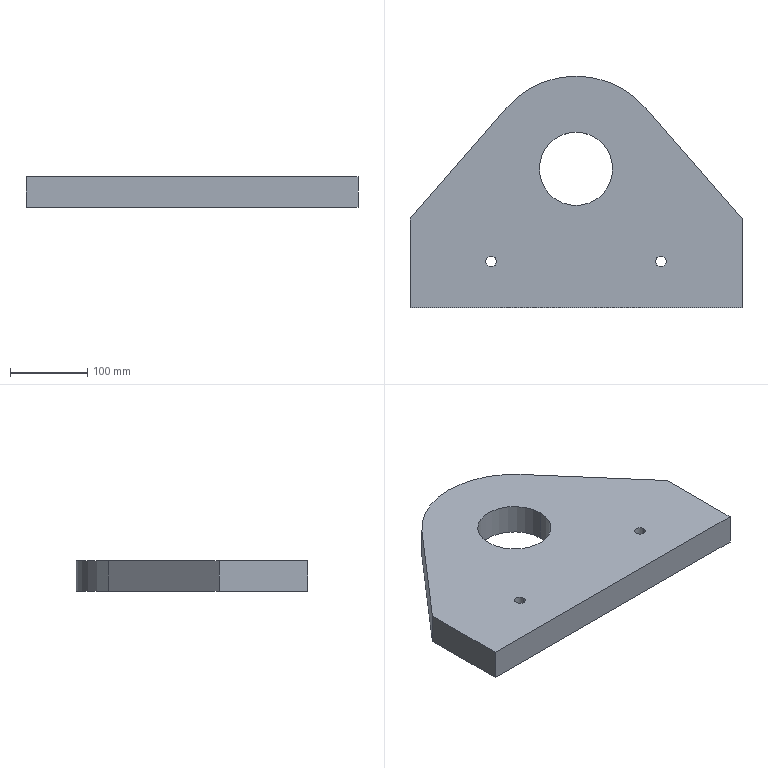Part | SolidWorks | features Extrusion 1, HoleWzd 1, ICE 1 | 1 solid | 14 faces | box 430 x 300 x 40 mm | volume 3646282 mm3 | cylinder 7 | plane 7 | commonest cylinder face diameters 14 x4 95 x2 240 x1
STEP:
#1=CARTESIAN_POINT('',(-117.,-120.,0.));
#2=VERTEX_POINT('',#1);
#3=CARTESIAN_POINT('',(-103.,-120.,0.));
#4=VERTEX_POINT('',#3);
#5=CARTESIAN_POINT('',(-110.,-120.,0.));
#6=DIRECTION('',(0.,0.,1.));
#7=DIRECTION('',(1.,0.,0.));
#8=AXIS2_PLACEMENT_3D('',#5,#6,#7);
#9=CIRCLE('',#8,7.);
#10=EDGE_CURVE('',#2,#4,#9,.T.);
#11=ORIENTED_EDGE('',*,*,#10,.F.);
#12=CARTESIAN_POINT('',(-117.,-120.,40.));
#13=VERTEX_POINT('',#12);
#14=CARTESIAN_POINT('',(-117.,-120.,40.));
#15=DIRECTION('',(0.,0.,1.));
#16=VECTOR('',#15,1000.);
#17=LINE('',#14,#16);
#18=EDGE_CURVE('',#2,#13,#17,.T.);
#19=ORIENTED_EDGE('',*,*,#18,.T.);
#20=CARTESIAN_POINT('',(-103.,-120.,40.));
#21=VERTEX_POINT('',#20);
#22=CARTESIAN_POINT('',(-110.,-120.,40.));
#23=DIRECTION('',(0.,0.,1.));
#24=DIRECTION('',(1.,0.,0.));
#25=AXIS2_PLACEMENT_3D('',#22,#23,#24);
#26=CIRCLE('',#25,7.);
#27=EDGE_CURVE('',#13,#21,#26,.T.);
#28=ORIENTED_EDGE('',*,*,#27,.T.);
#29=CARTESIAN_POINT('',(-103.,-120.,40.));
#30=DIRECTION('',(0.,0.,1.));
#31=VECTOR('',#30,1000.);
#32=LINE('',#29,#31);
#33=EDGE_CURVE('',#4,#21,#32,.T.);
#34=ORIENTED_EDGE('',*,*,#33,.F.);
#35=EDGE_LOOP('',(#11,#19,#28,#34));
#36=FACE_OUTER_BOUND('',#35,.T.);
#37=CARTESIAN_POINT('',(-110.,-120.,40.));
#38=DIRECTION('',(0.,0.,1.));
#39=DIRECTION('',(1.,0.,0.));
#40=AXIS2_PLACEMENT_3D('',#37,#38,#39);
#41=CYLINDRICAL_SURFACE('',#40,7.);
#42=ADVANCED_FACE('',(#36),#41,.F.);
#43=CARTESIAN_POINT('',(103.,-120.,0.));
#44=VERTEX_POINT('',#43);
#45=CARTESIAN_POINT('',(117.,-120.,0.));
#46=VERTEX_POINT('',#45);
#47=CARTESIAN_POINT('',(110.,-120.,0.));
#48=DIRECTION('',(0.,0.,1.));
#49=DIRECTION('',(1.,0.,0.));
#50=AXIS2_PLACEMENT_3D('',#47,#48,#49);
#51=CIRCLE('',#50,7.);
#52=EDGE_CURVE('',#44,#46,#51,.T.);
#53=ORIENTED_EDGE('',*,*,#52,.F.);
#54=CARTESIAN_POINT('',(103.,-120.,40.));
#55=VERTEX_POINT('',#54);
#56=CARTESIAN_POINT('',(103.,-120.,40.));
#57=DIRECTION('',(0.,0.,1.));
#58=VECTOR('',#57,1000.);
#59=LINE('',#56,#58);
#60=EDGE_CURVE('',#44,#55,#59,.T.);
#61=ORIENTED_EDGE('',*,*,#60,.T.);
#62=CARTESIAN_POINT('',(117.,-120.,40.));
#63=VERTEX_POINT('',#62);
#64=CARTESIAN_POINT('',(110.,-120.,40.));
#65=DIRECTION('',(0.,0.,1.));
#66=DIRECTION('',(1.,0.,0.));
#67=AXIS2_PLACEMENT_3D('',#64,#65,#66);
#68=CIRCLE('',#67,7.);
#69=EDGE_CURVE('',#55,#63,#68,.T.);
#70=ORIENTED_EDGE('',*,*,#69,.T.);
#71=CARTESIAN_POINT('',(117.,-120.,40.));
#72=DIRECTION('',(0.,0.,1.));
#73=VECTOR('',#72,1000.);
#74=LINE('',#71,#73);
#75=EDGE_CURVE('',#46,#63,#74,.T.);
#76=ORIENTED_EDGE('',*,*,#75,.F.);
#77=EDGE_LOOP('',(#53,#61,#70,#76));
#78=FACE_OUTER_BOUND('',#77,.T.);
#79=CARTESIAN_POINT('',(110.,-120.,40.));
#80=DIRECTION('',(0.,0.,1.));
#81=DIRECTION('',(1.,0.,0.));
#82=AXIS2_PLACEMENT_3D('',#79,#80,#81);
#83=CYLINDRICAL_SURFACE('',#82,7.);
#84=ADVANCED_FACE('',(#78),#83,.F.);
#85=CARTESIAN_POINT('',(-47.5,0.,0.));
#86=VERTEX_POINT('',#85);
#87=CARTESIAN_POINT('',(47.5,0.,0.));
#88=VERTEX_POINT('',#87);
#89=CARTESIAN_POINT('',(0.,0.,0.));
#90=DIRECTION('',(0.,0.,1.));
#91=DIRECTION('',(1.,0.,0.));
#92=AXIS2_PLACEMENT_3D('',#89,#90,#91);
#93=CIRCLE('',#92,47.5);
#94=EDGE_CURVE('',#86,#88,#93,.T.);
#95=ORIENTED_EDGE('',*,*,#94,.F.);
#96=CARTESIAN_POINT('',(-47.5,0.,40.));
#97=VERTEX_POINT('',#96);
#98=CARTESIAN_POINT('',(-47.5,0.,0.));
#99=DIRECTION('',(0.,0.,1.));
#100=VECTOR('',#99,1000.);
#101=LINE('',#98,#100);
#102=EDGE_CURVE('',#86,#97,#101,.T.);
#103=ORIENTED_EDGE('',*,*,#102,.T.);
#104=CARTESIAN_POINT('',(47.5,0.,40.));
#105=VERTEX_POINT('',#104);
#106=CARTESIAN_POINT('',(0.,0.,40.));
#107=DIRECTION('',(0.,0.,1.));
#108=DIRECTION('',(1.,0.,0.));
#109=AXIS2_PLACEMENT_3D('',#106,#107,#108);
#110=CIRCLE('',#109,47.5);
#111=EDGE_CURVE('',#97,#105,#110,.T.);
#112=ORIENTED_EDGE('',*,*,#111,.T.);
#113=CARTESIAN_POINT('',(47.5,0.,0.));
#114=DIRECTION('',(0.,0.,1.));
#115=VECTOR('',#114,1000.);
#116=LINE('',#113,#115);
#117=EDGE_CURVE('',#88,#105,#116,.T.);
#118=ORIENTED_EDGE('',*,*,#117,.F.);
#119=EDGE_LOOP('',(#95,#103,#112,#118));
#120=FACE_OUTER_BOUND('',#119,.T.);
#121=CARTESIAN_POINT('',(0.,0.,0.));
#122=DIRECTION('',(0.,0.,1.));
#123=DIRECTION('',(1.,0.,0.));
#124=AXIS2_PLACEMENT_3D('',#121,#122,#123);
#125=CYLINDRICAL_SURFACE('',#124,47.5);
#126=ADVANCED_FACE('',(#120),#125,.F.);
#127=CARTESIAN_POINT('',(90.723,78.545,0.));
#128=VERTEX_POINT('',#127);
#129=CARTESIAN_POINT('',(215.,-65.,0.));
#130=VERTEX_POINT('',#129);
#131=CARTESIAN_POINT('',(90.723,78.545,0.));
#132=DIRECTION('',(0.6545,-0.756,0.));
#133=VECTOR('',#132,1000.);
#134=LINE('',#131,#133);
#135=EDGE_CURVE('',#128,#130,#134,.T.);
#136=ORIENTED_EDGE('',*,*,#135,.F.);
#137=CARTESIAN_POINT('',(90.723,78.545,40.));
#138=VERTEX_POINT('',#137);
#139=CARTESIAN_POINT('',(90.723,78.545,40.));
#140=DIRECTION('',(0.,0.,-1.));
#141=VECTOR('',#140,1000.);
#142=LINE('',#139,#141);
#143=EDGE_CURVE('',#138,#128,#142,.T.);
#144=ORIENTED_EDGE('',*,*,#143,.F.);
#145=CARTESIAN_POINT('',(215.,-65.,40.));
#146=VERTEX_POINT('',#145);
#147=CARTESIAN_POINT('',(90.723,78.545,40.));
#148=DIRECTION('',(0.6545,-0.756,0.));
#149=VECTOR('',#148,1000.);
#150=LINE('',#147,#149);
#151=EDGE_CURVE('',#138,#146,#150,.T.);
#152=ORIENTED_EDGE('',*,*,#151,.T.);
#153=CARTESIAN_POINT('',(215.,-65.,40.));
#154=DIRECTION('',(0.,0.,-1.));
#155=VECTOR('',#154,1000.);
#156=LINE('',#153,#155);
#157=EDGE_CURVE('',#146,#130,#156,.T.);
#158=ORIENTED_EDGE('',*,*,#157,.T.);
#159=EDGE_LOOP('',(#136,#144,#152,#158));
#160=FACE_OUTER_BOUND('',#159,.T.);
#161=CARTESIAN_POINT('',(90.723,78.545,40.));
#162=DIRECTION('',(0.756,0.6545,0.));
#163=DIRECTION('',(-0.6545,0.756,0.));
#164=AXIS2_PLACEMENT_3D('',#161,#162,#163);
#165=PLANE('',#164);
#166=ADVANCED_FACE('',(#160),#165,.T.);
#167=CARTESIAN_POINT('',(-90.723,78.545,0.));
#168=VERTEX_POINT('',#167);
#169=CARTESIAN_POINT('',(0.,0.,0.));
#170=DIRECTION('',(0.,0.,1.));
#171=DIRECTION('',(1.,0.,0.));
#172=AXIS2_PLACEMENT_3D('',#169,#170,#171);
#173=CIRCLE('',#172,120.);
#174=EDGE_CURVE('',#128,#168,#173,.T.);
#175=ORIENTED_EDGE('',*,*,#174,.T.);
#176=CARTESIAN_POINT('',(-90.723,78.545,40.));
#177=VERTEX_POINT('',#176);
#178=CARTESIAN_POINT('',(-90.723,78.545,40.));
#179=DIRECTION('',(0.,0.,-1.));
#180=VECTOR('',#179,1000.);
#181=LINE('',#178,#180);
#182=EDGE_CURVE('',#177,#168,#181,.T.);
#183=ORIENTED_EDGE('',*,*,#182,.F.);
#184=CARTESIAN_POINT('',(0.,0.,40.));
#185=DIRECTION('',(0.,0.,1.));
#186=DIRECTION('',(1.,0.,0.));
#187=AXIS2_PLACEMENT_3D('',#184,#185,#186);
#188=CIRCLE('',#187,120.);
#189=EDGE_CURVE('',#138,#177,#188,.T.);
#190=ORIENTED_EDGE('',*,*,#189,.F.);
#191=ORIENTED_EDGE('',*,*,#143,.T.);
#192=EDGE_LOOP('',(#175,#183,#190,#191));
#193=FACE_OUTER_BOUND('',#192,.T.);
#194=CARTESIAN_POINT('',(0.,0.,40.));
#195=DIRECTION('',(0.,0.,-1.));
#196=DIRECTION('',(-1.,0.,0.));
#197=AXIS2_PLACEMENT_3D('',#194,#195,#196);
#198=CYLINDRICAL_SURFACE('',#197,120.);
#199=ADVANCED_FACE('',(#193),#198,.T.);
#200=CARTESIAN_POINT('',(-215.,-65.,0.));
#201=VERTEX_POINT('',#200);
#202=CARTESIAN_POINT('',(-90.723,78.545,0.));
#203=DIRECTION('',(-0.6545,-0.756,0.));
#204=VECTOR('',#203,1000.);
#205=LINE('',#202,#204);
#206=EDGE_CURVE('',#168,#201,#205,.T.);
#207=ORIENTED_EDGE('',*,*,#206,.T.);
#208=CARTESIAN_POINT('',(-215.,-65.,40.));
#209=VERTEX_POINT('',#208);
#210=CARTESIAN_POINT('',(-215.,-65.,40.));
#211=DIRECTION('',(0.,0.,-1.));
#212=VECTOR('',#211,1000.);
#213=LINE('',#210,#212);
#214=EDGE_CURVE('',#209,#201,#213,.T.);
#215=ORIENTED_EDGE('',*,*,#214,.F.);
#216=CARTESIAN_POINT('',(-90.723,78.545,40.));
#217=DIRECTION('',(-0.6545,-0.756,0.));
#218=VECTOR('',#217,1000.);
#219=LINE('',#216,#218);
#220=EDGE_CURVE('',#177,#209,#219,.T.);
#221=ORIENTED_EDGE('',*,*,#220,.F.);
#222=ORIENTED_EDGE('',*,*,#182,.T.);
#223=EDGE_LOOP('',(#207,#215,#221,#222));
#224=FACE_OUTER_BOUND('',#223,.T.);
#225=CARTESIAN_POINT('',(-90.723,78.545,40.));
#226=DIRECTION('',(0.756,-0.6545,0.));
#227=DIRECTION('',(0.6545,0.756,0.));
#228=AXIS2_PLACEMENT_3D('',#225,#226,#227);
#229=PLANE('',#228);
#230=ADVANCED_FACE('',(#224),#229,.F.);
#231=CARTESIAN_POINT('',(-215.,-180.,0.));
#232=VERTEX_POINT('',#231);
#233=CARTESIAN_POINT('',(-215.,0.,0.));
#234=DIRECTION('',(0.,-1.,0.));
#235=VECTOR('',#234,1000.);
#236=LINE('',#233,#235);
#237=EDGE_CURVE('',#201,#232,#236,.T.);
#238=ORIENTED_EDGE('',*,*,#237,.T.);
#239=CARTESIAN_POINT('',(-215.,-180.,40.));
#240=VERTEX_POINT('',#239);
#241=CARTESIAN_POINT('',(-215.,-180.,40.));
#242=DIRECTION('',(0.,0.,-1.));
#243=VECTOR('',#242,1000.);
#244=LINE('',#241,#243);
#245=EDGE_CURVE('',#240,#232,#244,.T.);
#246=ORIENTED_EDGE('',*,*,#245,.F.);
#247=CARTESIAN_POINT('',(-215.,0.,40.));
#248=DIRECTION('',(0.,-1.,0.));
#249=VECTOR('',#248,1000.);
#250=LINE('',#247,#249);
#251=EDGE_CURVE('',#209,#240,#250,.T.);
#252=ORIENTED_EDGE('',*,*,#251,.F.);
#253=ORIENTED_EDGE('',*,*,#214,.T.);
#254=EDGE_LOOP('',(#238,#246,#252,#253));
#255=FACE_OUTER_BOUND('',#254,.T.);
#256=CARTESIAN_POINT('',(-215.,0.,40.));
#257=DIRECTION('',(1.,0.,0.));
#258=DIRECTION('',(0.,0.,-1.));
#259=AXIS2_PLACEMENT_3D('',#256,#257,#258);
#260=PLANE('',#259);
#261=ADVANCED_FACE('',(#255),#260,.F.);
#262=CARTESIAN_POINT('',(215.,-180.,0.));
#263=VERTEX_POINT('',#262);
#264=CARTESIAN_POINT('',(0.,-180.,0.));
#265=DIRECTION('',(1.,0.,0.));
#266=VECTOR('',#265,1000.);
#267=LINE('',#264,#266);
#268=EDGE_CURVE('',#232,#263,#267,.T.);
#269=ORIENTED_EDGE('',*,*,#268,.T.);
#270=CARTESIAN_POINT('',(215.,-180.,40.));
#271=VERTEX_POINT('',#270);
#272=CARTESIAN_POINT('',(215.,-180.,40.));
#273=DIRECTION('',(0.,0.,-1.));
#274=VECTOR('',#273,1000.);
#275=LINE('',#272,#274);
#276=EDGE_CURVE('',#271,#263,#275,.T.);
#277=ORIENTED_EDGE('',*,*,#276,.F.);
#278=CARTESIAN_POINT('',(0.,-180.,40.));
#279=DIRECTION('',(1.,0.,0.));
#280=VECTOR('',#279,1000.);
#281=LINE('',#278,#280);
#282=EDGE_CURVE('',#240,#271,#281,.T.);
#283=ORIENTED_EDGE('',*,*,#282,.F.);
#284=ORIENTED_EDGE('',*,*,#245,.T.);
#285=EDGE_LOOP('',(#269,#277,#283,#284));
#286=FACE_OUTER_BOUND('',#285,.T.);
#287=CARTESIAN_POINT('',(0.,-180.,40.));
#288=DIRECTION('',(0.,1.,0.));
#289=DIRECTION('',(-1.,0.,0.));
#290=AXIS2_PLACEMENT_3D('',#287,#288,#289);
#291=PLANE('',#290);
#292=ADVANCED_FACE('',(#286),#291,.F.);
#293=CARTESIAN_POINT('',(215.,0.,0.));
#294=DIRECTION('',(0.,-1.,0.));
#295=VECTOR('',#294,1000.);
#296=LINE('',#293,#295);
#297=EDGE_CURVE('',#130,#263,#296,.T.);
#298=ORIENTED_EDGE('',*,*,#297,.F.);
#299=ORIENTED_EDGE('',*,*,#157,.F.);
#300=CARTESIAN_POINT('',(215.,0.,40.));
#301=DIRECTION('',(0.,-1.,0.));
#302=VECTOR('',#301,1000.);
#303=LINE('',#300,#302);
#304=EDGE_CURVE('',#146,#271,#303,.T.);
#305=ORIENTED_EDGE('',*,*,#304,.T.);
#306=ORIENTED_EDGE('',*,*,#276,.T.);
#307=EDGE_LOOP('',(#298,#299,#305,#306));
#308=FACE_OUTER_BOUND('',#307,.T.);
#309=CARTESIAN_POINT('',(215.,0.,40.));
#310=DIRECTION('',(1.,0.,0.));
#311=DIRECTION('',(0.,1.,0.));
#312=AXIS2_PLACEMENT_3D('',#309,#310,#311);
#313=PLANE('',#312);
#314=ADVANCED_FACE('',(#308),#313,.T.);
#315=CARTESIAN_POINT('',(-110.,-120.,40.));
#316=DIRECTION('',(0.,0.,1.));
#317=DIRECTION('',(1.,0.,0.));
#318=AXIS2_PLACEMENT_3D('',#315,#316,#317);
#319=CIRCLE('',#318,7.);
#320=EDGE_CURVE('',#21,#13,#319,.T.);
#321=ORIENTED_EDGE('',*,*,#320,.F.);
#322=ORIENTED_EDGE('',*,*,#27,.F.);
#323=EDGE_LOOP('',(#321,#322));
#324=FACE_BOUND('',#323,.T.);
#325=CARTESIAN_POINT('',(110.,-120.,40.));
#326=DIRECTION('',(0.,0.,1.));
#327=DIRECTION('',(1.,0.,0.));
#328=AXIS2_PLACEMENT_3D('',#325,#326,#327);
#329=CIRCLE('',#328,7.);
#330=EDGE_CURVE('',#63,#55,#329,.T.);
#331=ORIENTED_EDGE('',*,*,#330,.F.);
#332=ORIENTED_EDGE('',*,*,#69,.F.);
#333=EDGE_LOOP('',(#331,#332));
#334=FACE_BOUND('',#333,.T.);
#335=CARTESIAN_POINT('',(0.,0.,40.));
#336=DIRECTION('',(0.,0.,1.));
#337=DIRECTION('',(1.,0.,0.));
#338=AXIS2_PLACEMENT_3D('',#335,#336,#337);
#339=CIRCLE('',#338,47.5);
#340=EDGE_CURVE('',#105,#97,#339,.T.);
#341=ORIENTED_EDGE('',*,*,#340,.F.);
#342=ORIENTED_EDGE('',*,*,#111,.F.);
#343=EDGE_LOOP('',(#341,#342));
#344=FACE_BOUND('',#343,.T.);
#345=ORIENTED_EDGE('',*,*,#151,.F.);
#346=ORIENTED_EDGE('',*,*,#189,.T.);
#347=ORIENTED_EDGE('',*,*,#220,.T.);
#348=ORIENTED_EDGE('',*,*,#251,.T.);
#349=ORIENTED_EDGE('',*,*,#282,.T.);
#350=ORIENTED_EDGE('',*,*,#304,.F.);
#351=EDGE_LOOP('',(#345,#346,#347,#348,#349,#350));
#352=FACE_OUTER_BOUND('',#351,.T.);
#353=CARTESIAN_POINT('',(0.,0.,40.));
#354=DIRECTION('',(0.,0.,1.));
#355=DIRECTION('',(1.,0.,0.));
#356=AXIS2_PLACEMENT_3D('',#353,#354,#355);
#357=PLANE('',#356);
#358=ADVANCED_FACE('',(#324,#334,#344,#352),#357,.T.);
#359=CARTESIAN_POINT('',(-110.,-120.,0.));
#360=DIRECTION('',(0.,0.,1.));
#361=DIRECTION('',(1.,0.,0.));
#362=AXIS2_PLACEMENT_3D('',#359,#360,#361);
#363=CIRCLE('',#362,7.);
#364=EDGE_CURVE('',#4,#2,#363,.T.);
#365=ORIENTED_EDGE('',*,*,#364,.T.);
#366=ORIENTED_EDGE('',*,*,#10,.T.);
#367=EDGE_LOOP('',(#365,#366));
#368=FACE_BOUND('',#367,.T.);
#369=CARTESIAN_POINT('',(110.,-120.,0.));
#370=DIRECTION('',(0.,0.,1.));
#371=DIRECTION('',(1.,0.,0.));
#372=AXIS2_PLACEMENT_3D('',#369,#370,#371);
#373=CIRCLE('',#372,7.);
#374=EDGE_CURVE('',#46,#44,#373,.T.);
#375=ORIENTED_EDGE('',*,*,#374,.T.);
#376=ORIENTED_EDGE('',*,*,#52,.T.);
#377=EDGE_LOOP('',(#375,#376));
#378=FACE_BOUND('',#377,.T.);
#379=CARTESIAN_POINT('',(0.,0.,0.));
#380=DIRECTION('',(0.,0.,1.));
#381=DIRECTION('',(1.,0.,0.));
#382=AXIS2_PLACEMENT_3D('',#379,#380,#381);
#383=CIRCLE('',#382,47.5);
#384=EDGE_CURVE('',#88,#86,#383,.T.);
#385=ORIENTED_EDGE('',*,*,#384,.T.);
#386=ORIENTED_EDGE('',*,*,#94,.T.);
#387=EDGE_LOOP('',(#385,#386));
#388=FACE_BOUND('',#387,.T.);
#389=ORIENTED_EDGE('',*,*,#135,.T.);
#390=ORIENTED_EDGE('',*,*,#297,.T.);
#391=ORIENTED_EDGE('',*,*,#268,.F.);
#392=ORIENTED_EDGE('',*,*,#237,.F.);
#393=ORIENTED_EDGE('',*,*,#206,.F.);
#394=ORIENTED_EDGE('',*,*,#174,.F.);
#395=EDGE_LOOP('',(#389,#390,#391,#392,#393,#394));
#396=FACE_OUTER_BOUND('',#395,.T.);
#397=CARTESIAN_POINT('',(0.,0.,0.));
#398=DIRECTION('',(0.,0.,1.));
#399=DIRECTION('',(1.,0.,0.));
#400=AXIS2_PLACEMENT_3D('',#397,#398,#399);
#401=PLANE('',#400);
#402=ADVANCED_FACE('',(#368,#378,#388,#396),#401,.F.);
#403=ORIENTED_EDGE('',*,*,#102,.F.);
#404=ORIENTED_EDGE('',*,*,#384,.F.);
#405=ORIENTED_EDGE('',*,*,#117,.T.);
#406=ORIENTED_EDGE('',*,*,#340,.T.);
#407=EDGE_LOOP('',(#403,#404,#405,#406));
#408=FACE_OUTER_BOUND('',#407,.T.);
#409=CARTESIAN_POINT('',(0.,0.,0.));
#410=DIRECTION('',(0.,0.,1.));
#411=DIRECTION('',(1.,0.,0.));
#412=AXIS2_PLACEMENT_3D('',#409,#410,#411);
#413=CYLINDRICAL_SURFACE('',#412,47.5);
#414=ADVANCED_FACE('',(#408),#413,.F.);
#415=ORIENTED_EDGE('',*,*,#60,.F.);
#416=ORIENTED_EDGE('',*,*,#374,.F.);
#417=ORIENTED_EDGE('',*,*,#75,.T.);
#418=ORIENTED_EDGE('',*,*,#330,.T.);
#419=EDGE_LOOP('',(#415,#416,#417,#418));
#420=FACE_OUTER_BOUND('',#419,.T.);
#421=CARTESIAN_POINT('',(110.,-120.,40.));
#422=DIRECTION('',(0.,0.,1.));
#423=DIRECTION('',(1.,0.,0.));
#424=AXIS2_PLACEMENT_3D('',#421,#422,#423);
#425=CYLINDRICAL_SURFACE('',#424,7.);
#426=ADVANCED_FACE('',(#420),#425,.F.);
#427=ORIENTED_EDGE('',*,*,#18,.F.);
#428=ORIENTED_EDGE('',*,*,#364,.F.);
#429=ORIENTED_EDGE('',*,*,#33,.T.);
#430=ORIENTED_EDGE('',*,*,#320,.T.);
#431=EDGE_LOOP('',(#427,#428,#429,#430));
#432=FACE_OUTER_BOUND('',#431,.T.);
#433=CARTESIAN_POINT('',(-110.,-120.,40.));
#434=DIRECTION('',(0.,0.,1.));
#435=DIRECTION('',(1.,0.,0.));
#436=AXIS2_PLACEMENT_3D('',#433,#434,#435);
#437=CYLINDRICAL_SURFACE('',#436,7.);
#438=ADVANCED_FACE('',(#432),#437,.F.);
#439=CLOSED_SHELL('',(#42,#84,#126,#166,#199,#230,#261,#292,#314,#358,#402,#414,#426,#438));
#440=MANIFOLD_SOLID_BREP('',#439);
#441=CARTESIAN_POINT('',(0.,0.,0.));
#442=DIRECTION('',(0.,0.,1.));
#443=DIRECTION('',(1.,0.,0.));
#444=AXIS2_PLACEMENT_3D('',#441,#442,#443);
#445=(LENGTH_UNIT()NAMED_UNIT(*)SI_UNIT(.MILLI.,.METRE.));
#446=UNCERTAINTY_MEASURE_WITH_UNIT(LENGTH_MEASURE(0.00001),#445,'','');
#447=(NAMED_UNIT(*)PLANE_ANGLE_UNIT()SI_UNIT($,.RADIAN.));
#448=(NAMED_UNIT(*)SI_UNIT($,.STERADIAN.)SOLID_ANGLE_UNIT());
#449=(GEOMETRIC_REPRESENTATION_CONTEXT(3)GLOBAL_UNCERTAINTY_ASSIGNED_CONTEXT((#446))GLOBAL_UNIT_ASSIGNED_CONTEXT((#445,#447,#448))REPRESENTATION_CONTEXT('',''));
#450=ADVANCED_BREP_SHAPE_REPRESENTATION('',(#440,#444),#449);